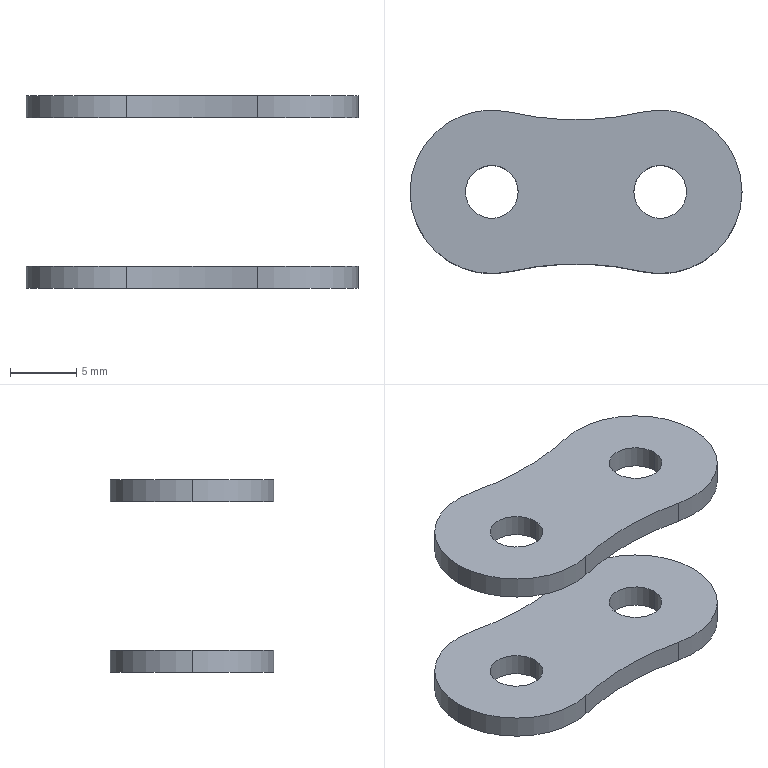Part | SolidWorks | 2 solids | 22 faces | box 25.03 x 12.33 x 14.51 mm | volume 799.359 mm3 | cylinder 18 | plane 4 | commonest cylinder face diameters 3.98 x8 12.33 x6 43.376 x4